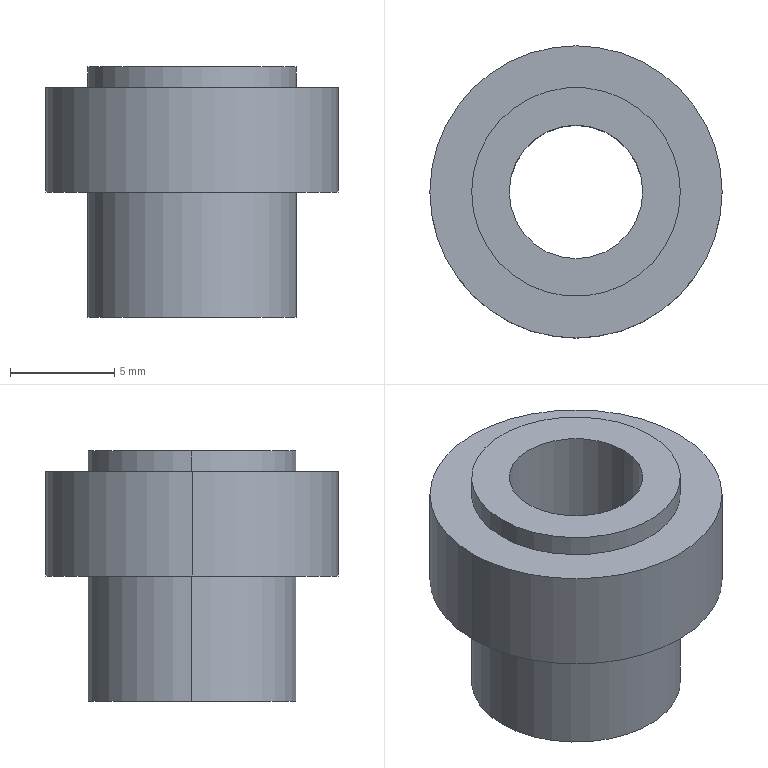Part | SolidWorks | features Extrusion 1, ICE 1 | 1 solid | 12 faces | box 14 x 14 x 12 mm | volume 933.43 mm3 | cylinder 8 | plane 4 | commonest cylinder face diameters 10 x4 6.4 x2 14 x2
STEP:
#1=CARTESIAN_POINT('',(7.,0.,5.));
#2=VERTEX_POINT('',#1);
#3=CARTESIAN_POINT('',(-7.,0.,5.));
#4=VERTEX_POINT('',#3);
#5=CARTESIAN_POINT('',(0.,0.,5.));
#6=DIRECTION('',(0.,0.,1.));
#7=DIRECTION('',(1.,0.,0.));
#8=AXIS2_PLACEMENT_3D('',#5,#6,#7);
#9=CIRCLE('',#8,7.);
#10=EDGE_CURVE('',#2,#4,#9,.T.);
#11=ORIENTED_EDGE('',*,*,#10,.F.);
#12=CARTESIAN_POINT('',(7.,0.,0.));
#13=VERTEX_POINT('',#12);
#14=CARTESIAN_POINT('',(7.,0.,5.));
#15=DIRECTION('',(0.,0.,-1.));
#16=VECTOR('',#15,1000.);
#17=LINE('',#14,#16);
#18=EDGE_CURVE('',#2,#13,#17,.T.);
#19=ORIENTED_EDGE('',*,*,#18,.T.);
#20=CARTESIAN_POINT('',(-7.,0.,0.));
#21=VERTEX_POINT('',#20);
#22=CARTESIAN_POINT('',(0.,0.,0.));
#23=DIRECTION('',(0.,0.,1.));
#24=DIRECTION('',(1.,0.,0.));
#25=AXIS2_PLACEMENT_3D('',#22,#23,#24);
#26=CIRCLE('',#25,7.);
#27=EDGE_CURVE('',#13,#21,#26,.T.);
#28=ORIENTED_EDGE('',*,*,#27,.T.);
#29=CARTESIAN_POINT('',(-7.,0.,5.));
#30=DIRECTION('',(0.,0.,-1.));
#31=VECTOR('',#30,1000.);
#32=LINE('',#29,#31);
#33=EDGE_CURVE('',#4,#21,#32,.T.);
#34=ORIENTED_EDGE('',*,*,#33,.F.);
#35=EDGE_LOOP('',(#11,#19,#28,#34));
#36=FACE_OUTER_BOUND('',#35,.T.);
#37=CARTESIAN_POINT('',(0.,0.,5.));
#38=DIRECTION('',(0.,0.,-1.));
#39=DIRECTION('',(-1.,0.,0.));
#40=AXIS2_PLACEMENT_3D('',#37,#38,#39);
#41=CYLINDRICAL_SURFACE('',#40,7.);
#42=ADVANCED_FACE('',(#36),#41,.T.);
#43=CARTESIAN_POINT('',(-3.2,0.,-6.));
#44=VERTEX_POINT('',#43);
#45=CARTESIAN_POINT('',(3.2,0.,-6.));
#46=VERTEX_POINT('',#45);
#47=CARTESIAN_POINT('',(0.,0.,-6.));
#48=DIRECTION('',(0.,0.,1.));
#49=DIRECTION('',(1.,0.,0.));
#50=AXIS2_PLACEMENT_3D('',#47,#48,#49);
#51=CIRCLE('',#50,3.2);
#52=EDGE_CURVE('',#44,#46,#51,.T.);
#53=ORIENTED_EDGE('',*,*,#52,.F.);
#54=CARTESIAN_POINT('',(-3.2,0.,6.));
#55=VERTEX_POINT('',#54);
#56=CARTESIAN_POINT('',(-3.2,0.,-6.));
#57=DIRECTION('',(0.,0.,1.));
#58=VECTOR('',#57,1000.);
#59=LINE('',#56,#58);
#60=EDGE_CURVE('',#44,#55,#59,.T.);
#61=ORIENTED_EDGE('',*,*,#60,.T.);
#62=CARTESIAN_POINT('',(3.2,0.,6.));
#63=VERTEX_POINT('',#62);
#64=CARTESIAN_POINT('',(0.,0.,6.));
#65=DIRECTION('',(0.,0.,1.));
#66=DIRECTION('',(1.,0.,0.));
#67=AXIS2_PLACEMENT_3D('',#64,#65,#66);
#68=CIRCLE('',#67,3.2);
#69=EDGE_CURVE('',#55,#63,#68,.T.);
#70=ORIENTED_EDGE('',*,*,#69,.T.);
#71=CARTESIAN_POINT('',(3.2,0.,-6.));
#72=DIRECTION('',(0.,0.,1.));
#73=VECTOR('',#72,1000.);
#74=LINE('',#71,#73);
#75=EDGE_CURVE('',#46,#63,#74,.T.);
#76=ORIENTED_EDGE('',*,*,#75,.F.);
#77=EDGE_LOOP('',(#53,#61,#70,#76));
#78=FACE_OUTER_BOUND('',#77,.T.);
#79=CARTESIAN_POINT('',(0.,0.,-6.));
#80=DIRECTION('',(0.,0.,1.));
#81=DIRECTION('',(1.,0.,0.));
#82=AXIS2_PLACEMENT_3D('',#79,#80,#81);
#83=CYLINDRICAL_SURFACE('',#82,3.2);
#84=ADVANCED_FACE('',(#78),#83,.F.);
#85=CARTESIAN_POINT('',(-5.,0.,5.));
#86=VERTEX_POINT('',#85);
#87=CARTESIAN_POINT('',(5.,0.,5.));
#88=VERTEX_POINT('',#87);
#89=CARTESIAN_POINT('',(0.,0.,5.));
#90=DIRECTION('',(0.,0.,-1.));
#91=DIRECTION('',(1.,0.,0.));
#92=AXIS2_PLACEMENT_3D('',#89,#90,#91);
#93=CIRCLE('',#92,5.);
#94=EDGE_CURVE('',#86,#88,#93,.T.);
#95=ORIENTED_EDGE('',*,*,#94,.F.);
#96=CARTESIAN_POINT('',(-5.,0.,6.));
#97=VERTEX_POINT('',#96);
#98=CARTESIAN_POINT('',(-5.,0.,-6.));
#99=DIRECTION('',(0.,0.,1.));
#100=VECTOR('',#99,1000.);
#101=LINE('',#98,#100);
#102=EDGE_CURVE('',#86,#97,#101,.T.);
#103=ORIENTED_EDGE('',*,*,#102,.T.);
#104=CARTESIAN_POINT('',(5.,0.,6.));
#105=VERTEX_POINT('',#104);
#106=CARTESIAN_POINT('',(0.,0.,6.));
#107=DIRECTION('',(0.,0.,1.));
#108=DIRECTION('',(1.,0.,0.));
#109=AXIS2_PLACEMENT_3D('',#106,#107,#108);
#110=CIRCLE('',#109,5.);
#111=EDGE_CURVE('',#105,#97,#110,.T.);
#112=ORIENTED_EDGE('',*,*,#111,.F.);
#113=CARTESIAN_POINT('',(5.,0.,-6.));
#114=DIRECTION('',(0.,0.,1.));
#115=VECTOR('',#114,1000.);
#116=LINE('',#113,#115);
#117=EDGE_CURVE('',#88,#105,#116,.T.);
#118=ORIENTED_EDGE('',*,*,#117,.F.);
#119=EDGE_LOOP('',(#95,#103,#112,#118));
#120=FACE_OUTER_BOUND('',#119,.T.);
#121=CARTESIAN_POINT('',(0.,0.,-6.));
#122=DIRECTION('',(0.,0.,1.));
#123=DIRECTION('',(1.,0.,0.));
#124=AXIS2_PLACEMENT_3D('',#121,#122,#123);
#125=CYLINDRICAL_SURFACE('',#124,5.);
#126=ADVANCED_FACE('',(#120),#125,.T.);
#127=CARTESIAN_POINT('',(5.,0.,-6.));
#128=VERTEX_POINT('',#127);
#129=CARTESIAN_POINT('',(-5.,0.,-6.));
#130=VERTEX_POINT('',#129);
#131=CARTESIAN_POINT('',(0.,0.,-6.));
#132=DIRECTION('',(0.,0.,1.));
#133=DIRECTION('',(1.,0.,0.));
#134=AXIS2_PLACEMENT_3D('',#131,#132,#133);
#135=CIRCLE('',#134,5.);
#136=EDGE_CURVE('',#128,#130,#135,.T.);
#137=ORIENTED_EDGE('',*,*,#136,.T.);
#138=CARTESIAN_POINT('',(-5.,0.,0.));
#139=VERTEX_POINT('',#138);
#140=CARTESIAN_POINT('',(-5.,0.,-6.));
#141=DIRECTION('',(0.,0.,1.));
#142=VECTOR('',#141,1000.);
#143=LINE('',#140,#142);
#144=EDGE_CURVE('',#130,#139,#143,.T.);
#145=ORIENTED_EDGE('',*,*,#144,.T.);
#146=CARTESIAN_POINT('',(5.,0.,0.));
#147=VERTEX_POINT('',#146);
#148=CARTESIAN_POINT('',(0.,0.,0.));
#149=DIRECTION('',(0.,0.,-1.));
#150=DIRECTION('',(1.,0.,0.));
#151=AXIS2_PLACEMENT_3D('',#148,#149,#150);
#152=CIRCLE('',#151,5.);
#153=EDGE_CURVE('',#139,#147,#152,.T.);
#154=ORIENTED_EDGE('',*,*,#153,.T.);
#155=CARTESIAN_POINT('',(5.,0.,-6.));
#156=DIRECTION('',(0.,0.,1.));
#157=VECTOR('',#156,1000.);
#158=LINE('',#155,#157);
#159=EDGE_CURVE('',#128,#147,#158,.T.);
#160=ORIENTED_EDGE('',*,*,#159,.F.);
#161=EDGE_LOOP('',(#137,#145,#154,#160));
#162=FACE_OUTER_BOUND('',#161,.T.);
#163=CARTESIAN_POINT('',(0.,0.,-6.));
#164=DIRECTION('',(0.,0.,1.));
#165=DIRECTION('',(1.,0.,0.));
#166=AXIS2_PLACEMENT_3D('',#163,#164,#165);
#167=CYLINDRICAL_SURFACE('',#166,5.);
#168=ADVANCED_FACE('',(#162),#167,.T.);
#169=ORIENTED_EDGE('',*,*,#144,.F.);
#170=CARTESIAN_POINT('',(0.,0.,-6.));
#171=DIRECTION('',(0.,0.,1.));
#172=DIRECTION('',(1.,0.,0.));
#173=AXIS2_PLACEMENT_3D('',#170,#171,#172);
#174=CIRCLE('',#173,5.);
#175=EDGE_CURVE('',#130,#128,#174,.T.);
#176=ORIENTED_EDGE('',*,*,#175,.T.);
#177=ORIENTED_EDGE('',*,*,#159,.T.);
#178=CARTESIAN_POINT('',(0.,0.,0.));
#179=DIRECTION('',(0.,0.,-1.));
#180=DIRECTION('',(1.,0.,0.));
#181=AXIS2_PLACEMENT_3D('',#178,#179,#180);
#182=CIRCLE('',#181,5.);
#183=EDGE_CURVE('',#147,#139,#182,.T.);
#184=ORIENTED_EDGE('',*,*,#183,.T.);
#185=EDGE_LOOP('',(#169,#176,#177,#184));
#186=FACE_OUTER_BOUND('',#185,.T.);
#187=CARTESIAN_POINT('',(0.,0.,-6.));
#188=DIRECTION('',(0.,0.,1.));
#189=DIRECTION('',(1.,0.,0.));
#190=AXIS2_PLACEMENT_3D('',#187,#188,#189);
#191=CYLINDRICAL_SURFACE('',#190,5.);
#192=ADVANCED_FACE('',(#186),#191,.T.);
#193=ORIENTED_EDGE('',*,*,#102,.F.);
#194=CARTESIAN_POINT('',(0.,0.,5.));
#195=DIRECTION('',(0.,0.,-1.));
#196=DIRECTION('',(1.,0.,0.));
#197=AXIS2_PLACEMENT_3D('',#194,#195,#196);
#198=CIRCLE('',#197,5.);
#199=EDGE_CURVE('',#88,#86,#198,.T.);
#200=ORIENTED_EDGE('',*,*,#199,.F.);
#201=ORIENTED_EDGE('',*,*,#117,.T.);
#202=CARTESIAN_POINT('',(0.,0.,6.));
#203=DIRECTION('',(0.,0.,1.));
#204=DIRECTION('',(1.,0.,0.));
#205=AXIS2_PLACEMENT_3D('',#202,#203,#204);
#206=CIRCLE('',#205,5.);
#207=EDGE_CURVE('',#97,#105,#206,.T.);
#208=ORIENTED_EDGE('',*,*,#207,.F.);
#209=EDGE_LOOP('',(#193,#200,#201,#208));
#210=FACE_OUTER_BOUND('',#209,.T.);
#211=CARTESIAN_POINT('',(0.,0.,-6.));
#212=DIRECTION('',(0.,0.,1.));
#213=DIRECTION('',(1.,0.,0.));
#214=AXIS2_PLACEMENT_3D('',#211,#212,#213);
#215=CYLINDRICAL_SURFACE('',#214,5.);
#216=ADVANCED_FACE('',(#210),#215,.T.);
#217=CARTESIAN_POINT('',(0.,0.,-6.));
#218=DIRECTION('',(0.,0.,1.));
#219=DIRECTION('',(1.,0.,0.));
#220=AXIS2_PLACEMENT_3D('',#217,#218,#219);
#221=CIRCLE('',#220,3.2);
#222=EDGE_CURVE('',#46,#44,#221,.T.);
#223=ORIENTED_EDGE('',*,*,#222,.T.);
#224=ORIENTED_EDGE('',*,*,#52,.T.);
#225=EDGE_LOOP('',(#223,#224));
#226=FACE_BOUND('',#225,.T.);
#227=ORIENTED_EDGE('',*,*,#136,.F.);
#228=ORIENTED_EDGE('',*,*,#175,.F.);
#229=EDGE_LOOP('',(#227,#228));
#230=FACE_OUTER_BOUND('',#229,.T.);
#231=CARTESIAN_POINT('',(0.,0.,-6.));
#232=DIRECTION('',(0.,0.,1.));
#233=DIRECTION('',(1.,0.,0.));
#234=AXIS2_PLACEMENT_3D('',#231,#232,#233);
#235=PLANE('',#234);
#236=ADVANCED_FACE('',(#226,#230),#235,.F.);
#237=CARTESIAN_POINT('',(0.,0.,6.));
#238=DIRECTION('',(0.,0.,1.));
#239=DIRECTION('',(1.,0.,0.));
#240=AXIS2_PLACEMENT_3D('',#237,#238,#239);
#241=CIRCLE('',#240,3.2);
#242=EDGE_CURVE('',#63,#55,#241,.T.);
#243=ORIENTED_EDGE('',*,*,#242,.F.);
#244=ORIENTED_EDGE('',*,*,#69,.F.);
#245=EDGE_LOOP('',(#243,#244));
#246=FACE_BOUND('',#245,.T.);
#247=ORIENTED_EDGE('',*,*,#111,.T.);
#248=ORIENTED_EDGE('',*,*,#207,.T.);
#249=EDGE_LOOP('',(#247,#248));
#250=FACE_OUTER_BOUND('',#249,.T.);
#251=CARTESIAN_POINT('',(0.,0.,6.));
#252=DIRECTION('',(0.,0.,1.));
#253=DIRECTION('',(1.,0.,0.));
#254=AXIS2_PLACEMENT_3D('',#251,#252,#253);
#255=PLANE('',#254);
#256=ADVANCED_FACE('',(#246,#250),#255,.T.);
#257=ORIENTED_EDGE('',*,*,#60,.F.);
#258=ORIENTED_EDGE('',*,*,#222,.F.);
#259=ORIENTED_EDGE('',*,*,#75,.T.);
#260=ORIENTED_EDGE('',*,*,#242,.T.);
#261=EDGE_LOOP('',(#257,#258,#259,#260));
#262=FACE_OUTER_BOUND('',#261,.T.);
#263=CARTESIAN_POINT('',(0.,0.,-6.));
#264=DIRECTION('',(0.,0.,1.));
#265=DIRECTION('',(1.,0.,0.));
#266=AXIS2_PLACEMENT_3D('',#263,#264,#265);
#267=CYLINDRICAL_SURFACE('',#266,3.2);
#268=ADVANCED_FACE('',(#262),#267,.F.);
#269=ORIENTED_EDGE('',*,*,#199,.T.);
#270=ORIENTED_EDGE('',*,*,#94,.T.);
#271=EDGE_LOOP('',(#269,#270));
#272=FACE_BOUND('',#271,.T.);
#273=CARTESIAN_POINT('',(0.,0.,5.));
#274=DIRECTION('',(0.,0.,1.));
#275=DIRECTION('',(1.,0.,0.));
#276=AXIS2_PLACEMENT_3D('',#273,#274,#275);
#277=CIRCLE('',#276,7.);
#278=EDGE_CURVE('',#4,#2,#277,.T.);
#279=ORIENTED_EDGE('',*,*,#278,.T.);
#280=ORIENTED_EDGE('',*,*,#10,.T.);
#281=EDGE_LOOP('',(#279,#280));
#282=FACE_OUTER_BOUND('',#281,.T.);
#283=CARTESIAN_POINT('',(0.,0.,5.));
#284=DIRECTION('',(0.,0.,1.));
#285=DIRECTION('',(1.,0.,0.));
#286=AXIS2_PLACEMENT_3D('',#283,#284,#285);
#287=PLANE('',#286);
#288=ADVANCED_FACE('',(#272,#282),#287,.T.);
#289=ORIENTED_EDGE('',*,*,#183,.F.);
#290=ORIENTED_EDGE('',*,*,#153,.F.);
#291=EDGE_LOOP('',(#289,#290));
#292=FACE_BOUND('',#291,.T.);
#293=CARTESIAN_POINT('',(0.,0.,0.));
#294=DIRECTION('',(0.,0.,1.));
#295=DIRECTION('',(1.,0.,0.));
#296=AXIS2_PLACEMENT_3D('',#293,#294,#295);
#297=CIRCLE('',#296,7.);
#298=EDGE_CURVE('',#21,#13,#297,.T.);
#299=ORIENTED_EDGE('',*,*,#298,.F.);
#300=ORIENTED_EDGE('',*,*,#27,.F.);
#301=EDGE_LOOP('',(#299,#300));
#302=FACE_OUTER_BOUND('',#301,.T.);
#303=CARTESIAN_POINT('',(0.,0.,0.));
#304=DIRECTION('',(0.,0.,1.));
#305=DIRECTION('',(1.,0.,0.));
#306=AXIS2_PLACEMENT_3D('',#303,#304,#305);
#307=PLANE('',#306);
#308=ADVANCED_FACE('',(#292,#302),#307,.F.);
#309=ORIENTED_EDGE('',*,*,#18,.F.);
#310=ORIENTED_EDGE('',*,*,#278,.F.);
#311=ORIENTED_EDGE('',*,*,#33,.T.);
#312=ORIENTED_EDGE('',*,*,#298,.T.);
#313=EDGE_LOOP('',(#309,#310,#311,#312));
#314=FACE_OUTER_BOUND('',#313,.T.);
#315=CARTESIAN_POINT('',(0.,0.,5.));
#316=DIRECTION('',(0.,0.,-1.));
#317=DIRECTION('',(-1.,0.,0.));
#318=AXIS2_PLACEMENT_3D('',#315,#316,#317);
#319=CYLINDRICAL_SURFACE('',#318,7.);
#320=ADVANCED_FACE('',(#314),#319,.T.);
#321=CLOSED_SHELL('',(#42,#84,#126,#168,#192,#216,#236,#256,#268,#288,#308,#320));
#322=MANIFOLD_SOLID_BREP('',#321);
#323=CARTESIAN_POINT('',(0.,0.,0.));
#324=DIRECTION('',(0.,0.,1.));
#325=DIRECTION('',(1.,0.,0.));
#326=AXIS2_PLACEMENT_3D('',#323,#324,#325);
#327=(LENGTH_UNIT()NAMED_UNIT(*)SI_UNIT(.MILLI.,.METRE.));
#328=UNCERTAINTY_MEASURE_WITH_UNIT(LENGTH_MEASURE(0.00001),#327,'','');
#329=(NAMED_UNIT(*)PLANE_ANGLE_UNIT()SI_UNIT($,.RADIAN.));
#330=(NAMED_UNIT(*)SI_UNIT($,.STERADIAN.)SOLID_ANGLE_UNIT());
#331=(GEOMETRIC_REPRESENTATION_CONTEXT(3)GLOBAL_UNCERTAINTY_ASSIGNED_CONTEXT((#328))GLOBAL_UNIT_ASSIGNED_CONTEXT((#327,#329,#330))REPRESENTATION_CONTEXT('',''));
#332=ADVANCED_BREP_SHAPE_REPRESENTATION('',(#322,#326),#331);